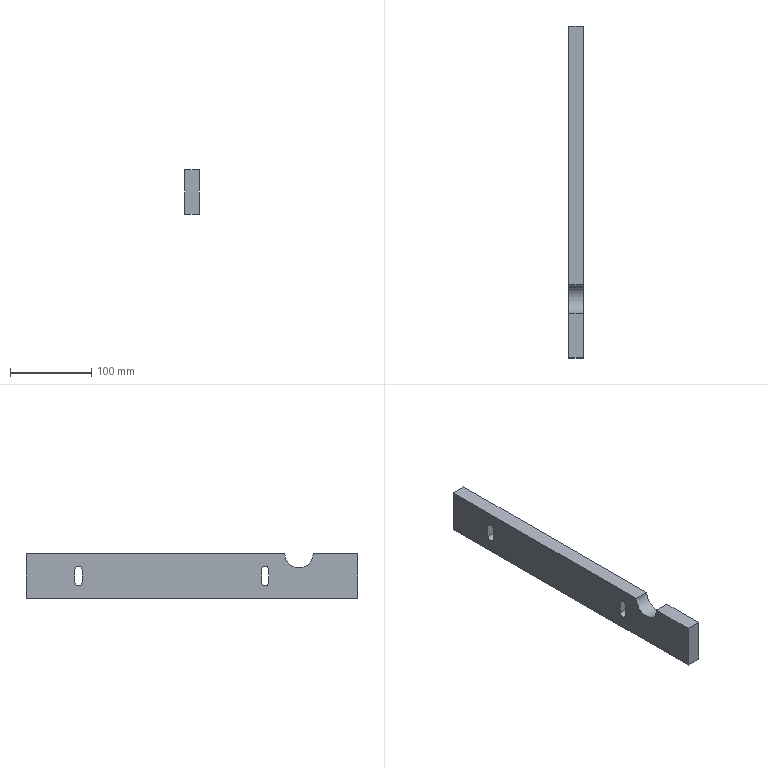Part | STEP file | Superstructure_3 | 1 solid | 16 faces | box 18 x 408 x 55 mm | volume 388111 mm3 | plane 11 | cylinder 5 | commonest cylinder face diameters 9 x4 35 x1
STEP:
#1=CARTESIAN_POINT('',(0.,0.,0.));
#2=DIRECTION('',(0.,0.,1.));
#3=DIRECTION('',(1.,0.,0.));
#4=AXIS2_PLACEMENT_3D('',#1,#2,#3);
#5=CARTESIAN_POINT('',(-9.,204.,27.5));
#6=VERTEX_POINT('',#5);
#7=CARTESIAN_POINT('',(-9.,204.,-27.5));
#8=VERTEX_POINT('',#7);
#9=CARTESIAN_POINT('',(-9.,204.,27.5));
#10=DIRECTION('',(0.,0.,-1.));
#11=VECTOR('',#10,1.);
#12=LINE('',#9,#11);
#13=CARTESIAN_POINT('',(-9.,204.,27.5));
#14=DIRECTION('',(1.,0.,0.));
#15=DIRECTION('',(0.,0.,-1.));
#16=AXIS2_PLACEMENT_3D('',#13,#14,#15);
#17=PLANE('',#16);
#18=CARTESIAN_POINT('',(0.,0.));
#19=DIRECTION('',(1.,0.));
#20=VECTOR('',#19,1.);
#21=LINE('',#18,#20);
#22=(GEOMETRIC_REPRESENTATION_CONTEXT(2)PARAMETRIC_REPRESENTATION_CONTEXT()REPRESENTATION_CONTEXT('',''));
#23=DEFINITIONAL_REPRESENTATION('',(#21),#22);
#24=PCURVE('',#17,#23);
#25=CARTESIAN_POINT('',(0.,204.,0.));
#26=DIRECTION('',(0.,1.,0.));
#27=DIRECTION('',(0.,0.,1.));
#28=AXIS2_PLACEMENT_3D('',#25,#26,#27);
#29=PLANE('',#28);
#30=CARTESIAN_POINT('',(27.5,-9.));
#31=DIRECTION('',(-1.,0.));
#32=VECTOR('',#31,1.);
#33=LINE('',#30,#32);
#34=(GEOMETRIC_REPRESENTATION_CONTEXT(2)PARAMETRIC_REPRESENTATION_CONTEXT()REPRESENTATION_CONTEXT('',''));
#35=DEFINITIONAL_REPRESENTATION('',(#33),#34);
#36=PCURVE('',#29,#35);
#37=SURFACE_CURVE('',#12,(#24,#36),.PCURVE_S1.);
#38=EDGE_CURVE('',#6,#8,#37,.T.);
#39=ORIENTED_EDGE('',*,*,#38,.F.);
#40=CARTESIAN_POINT('',(-9.,-114.,27.5));
#41=VERTEX_POINT('',#40);
#42=CARTESIAN_POINT('',(-9.,204.,27.5));
#43=DIRECTION('',(0.,-1.,0.));
#44=VECTOR('',#43,1.);
#45=LINE('',#42,#44);
#46=CARTESIAN_POINT('',(0.,0.));
#47=DIRECTION('',(0.,-1.));
#48=VECTOR('',#47,1.);
#49=LINE('',#46,#48);
#50=(GEOMETRIC_REPRESENTATION_CONTEXT(2)PARAMETRIC_REPRESENTATION_CONTEXT()REPRESENTATION_CONTEXT('',''));
#51=DEFINITIONAL_REPRESENTATION('',(#49),#50);
#52=PCURVE('',#17,#51);
#53=CARTESIAN_POINT('',(9.,204.,27.5));
#54=DIRECTION('',(0.,0.,-1.));
#55=DIRECTION('',(-1.,0.,0.));
#56=AXIS2_PLACEMENT_3D('',#53,#54,#55);
#57=PLANE('',#56);
#58=CARTESIAN_POINT('',(18.,0.));
#59=DIRECTION('',(0.,-1.));
#60=VECTOR('',#59,1.);
#61=LINE('',#58,#60);
#62=(GEOMETRIC_REPRESENTATION_CONTEXT(2)PARAMETRIC_REPRESENTATION_CONTEXT()REPRESENTATION_CONTEXT('',''));
#63=DEFINITIONAL_REPRESENTATION('',(#61),#62);
#64=PCURVE('',#57,#63);
#65=SURFACE_CURVE('',#45,(#52,#64),.PCURVE_S1.);
#66=EDGE_CURVE('',#6,#41,#65,.T.);
#67=ORIENTED_EDGE('',*,*,#66,.T.);
#68=CARTESIAN_POINT('',(-9.,-149.,27.5));
#69=VERTEX_POINT('',#68);
#70=CARTESIAN_POINT('',(-9.,-131.5,27.5));
#71=DIRECTION('',(1.,0.,0.));
#72=DIRECTION('',(0.,1.,0.));
#73=AXIS2_PLACEMENT_3D('',#70,#71,#72);
#74=CIRCLE('',#73,17.5);
#75=CARTESIAN_POINT('',(0.,-335.5));
#76=DIRECTION('',(0.,1.));
#77=AXIS2_PLACEMENT_2D('',#75,#76);
#78=CIRCLE('',#77,17.5);
#79=(GEOMETRIC_REPRESENTATION_CONTEXT(2)PARAMETRIC_REPRESENTATION_CONTEXT()REPRESENTATION_CONTEXT('',''));
#80=DEFINITIONAL_REPRESENTATION('',(#78),#79);
#81=PCURVE('',#17,#80);
#82=CARTESIAN_POINT('',(15.,-131.5,27.5));
#83=DIRECTION('',(1.,0.,0.));
#84=DIRECTION('',(0.,1.,0.));
#85=AXIS2_PLACEMENT_3D('',#82,#83,#84);
#86=CYLINDRICAL_SURFACE('',#85,17.5);
#87=CARTESIAN_POINT('',(0.,-24.));
#88=DIRECTION('',(1.,0.));
#89=VECTOR('',#88,1.);
#90=LINE('',#87,#89);
#91=(GEOMETRIC_REPRESENTATION_CONTEXT(2)PARAMETRIC_REPRESENTATION_CONTEXT()REPRESENTATION_CONTEXT('',''));
#92=DEFINITIONAL_REPRESENTATION('',(#90),#91);
#93=PCURVE('',#86,#92);
#94=SURFACE_CURVE('',#74,(#81,#93),.PCURVE_S1.);
#95=EDGE_CURVE('',#69,#41,#94,.T.);
#96=ORIENTED_EDGE('',*,*,#95,.F.);
#97=CARTESIAN_POINT('',(-9.,-204.,27.5));
#98=VERTEX_POINT('',#97);
#99=CARTESIAN_POINT('',(-9.,204.,27.5));
#100=DIRECTION('',(0.,-1.,0.));
#101=VECTOR('',#100,1.);
#102=LINE('',#99,#101);
#103=CARTESIAN_POINT('',(0.,0.));
#104=DIRECTION('',(0.,-1.));
#105=VECTOR('',#104,1.);
#106=LINE('',#103,#105);
#107=(GEOMETRIC_REPRESENTATION_CONTEXT(2)PARAMETRIC_REPRESENTATION_CONTEXT()REPRESENTATION_CONTEXT('',''));
#108=DEFINITIONAL_REPRESENTATION('',(#106),#107);
#109=PCURVE('',#17,#108);
#110=CARTESIAN_POINT('',(9.,204.,27.5));
#111=DIRECTION('',(0.,0.,-1.));
#112=DIRECTION('',(-1.,0.,0.));
#113=AXIS2_PLACEMENT_3D('',#110,#111,#112);
#114=PLANE('',#113);
#115=CARTESIAN_POINT('',(18.,0.));
#116=DIRECTION('',(0.,-1.));
#117=VECTOR('',#116,1.);
#118=LINE('',#115,#117);
#119=(GEOMETRIC_REPRESENTATION_CONTEXT(2)PARAMETRIC_REPRESENTATION_CONTEXT()REPRESENTATION_CONTEXT('',''));
#120=DEFINITIONAL_REPRESENTATION('',(#118),#119);
#121=PCURVE('',#114,#120);
#122=SURFACE_CURVE('',#102,(#109,#121),.PCURVE_S1.);
#123=EDGE_CURVE('',#69,#98,#122,.T.);
#124=ORIENTED_EDGE('',*,*,#123,.T.);
#125=CARTESIAN_POINT('',(-9.,-204.,-27.5));
#126=VERTEX_POINT('',#125);
#127=CARTESIAN_POINT('',(-9.,-204.,27.5));
#128=DIRECTION('',(0.,0.,-1.));
#129=VECTOR('',#128,1.);
#130=LINE('',#127,#129);
#131=CARTESIAN_POINT('',(0.,-408.));
#132=DIRECTION('',(1.,0.));
#133=VECTOR('',#132,1.);
#134=LINE('',#131,#133);
#135=(GEOMETRIC_REPRESENTATION_CONTEXT(2)PARAMETRIC_REPRESENTATION_CONTEXT()REPRESENTATION_CONTEXT('',''));
#136=DEFINITIONAL_REPRESENTATION('',(#134),#135);
#137=PCURVE('',#17,#136);
#138=CARTESIAN_POINT('',(0.,-204.,0.));
#139=DIRECTION('',(0.,1.,0.));
#140=DIRECTION('',(0.,0.,1.));
#141=AXIS2_PLACEMENT_3D('',#138,#139,#140);
#142=PLANE('',#141);
#143=CARTESIAN_POINT('',(27.5,-9.));
#144=DIRECTION('',(-1.,0.));
#145=VECTOR('',#144,1.);
#146=LINE('',#143,#145);
#147=(GEOMETRIC_REPRESENTATION_CONTEXT(2)PARAMETRIC_REPRESENTATION_CONTEXT()REPRESENTATION_CONTEXT('',''));
#148=DEFINITIONAL_REPRESENTATION('',(#146),#147);
#149=PCURVE('',#142,#148);
#150=SURFACE_CURVE('',#130,(#137,#149),.PCURVE_S1.);
#151=EDGE_CURVE('',#98,#126,#150,.T.);
#152=ORIENTED_EDGE('',*,*,#151,.T.);
#153=CARTESIAN_POINT('',(-9.,204.,-27.5));
#154=DIRECTION('',(0.,-1.,0.));
#155=VECTOR('',#154,1.);
#156=LINE('',#153,#155);
#157=CARTESIAN_POINT('',(55.,0.));
#158=DIRECTION('',(0.,-1.));
#159=VECTOR('',#158,1.);
#160=LINE('',#157,#159);
#161=(GEOMETRIC_REPRESENTATION_CONTEXT(2)PARAMETRIC_REPRESENTATION_CONTEXT()REPRESENTATION_CONTEXT('',''));
#162=DEFINITIONAL_REPRESENTATION('',(#160),#161);
#163=PCURVE('',#17,#162);
#164=CARTESIAN_POINT('',(-9.,204.,-27.5));
#165=DIRECTION('',(0.,0.,1.));
#166=DIRECTION('',(1.,0.,0.));
#167=AXIS2_PLACEMENT_3D('',#164,#165,#166);
#168=PLANE('',#167);
#169=CARTESIAN_POINT('',(0.,0.));
#170=DIRECTION('',(0.,-1.));
#171=VECTOR('',#170,1.);
#172=LINE('',#169,#171);
#173=(GEOMETRIC_REPRESENTATION_CONTEXT(2)PARAMETRIC_REPRESENTATION_CONTEXT()REPRESENTATION_CONTEXT('',''));
#174=DEFINITIONAL_REPRESENTATION('',(#172),#173);
#175=PCURVE('',#168,#174);
#176=SURFACE_CURVE('',#156,(#163,#175),.PCURVE_S1.);
#177=EDGE_CURVE('',#8,#126,#176,.T.);
#178=ORIENTED_EDGE('',*,*,#177,.F.);
#179=EDGE_LOOP('',(#39,#67,#96,#124,#152,#178));
#180=FACE_BOUND('',#179,.F.);
#181=CARTESIAN_POINT('',(-9.,-85.5,7.5));
#182=VERTEX_POINT('',#181);
#183=CARTESIAN_POINT('',(-9.,-94.5,7.5));
#184=VERTEX_POINT('',#183);
#185=CARTESIAN_POINT('',(-9.,-90.,7.5));
#186=DIRECTION('',(1.,0.,0.));
#187=DIRECTION('',(0.,1.,0.));
#188=AXIS2_PLACEMENT_3D('',#185,#186,#187);
#189=CIRCLE('',#188,4.5);
#190=CARTESIAN_POINT('',(20.,-294.));
#191=DIRECTION('',(0.,1.));
#192=AXIS2_PLACEMENT_2D('',#190,#191);
#193=CIRCLE('',#192,4.5);
#194=(GEOMETRIC_REPRESENTATION_CONTEXT(2)PARAMETRIC_REPRESENTATION_CONTEXT()REPRESENTATION_CONTEXT('',''));
#195=DEFINITIONAL_REPRESENTATION('',(#193),#194);
#196=PCURVE('',#17,#195);
#197=CARTESIAN_POINT('',(10.,-90.,7.5));
#198=DIRECTION('',(1.,0.,0.));
#199=DIRECTION('',(0.,1.,0.));
#200=AXIS2_PLACEMENT_3D('',#197,#198,#199);
#201=CYLINDRICAL_SURFACE('',#200,4.5);
#202=CARTESIAN_POINT('',(0.,-19.));
#203=DIRECTION('',(1.,0.));
#204=VECTOR('',#203,1.);
#205=LINE('',#202,#204);
#206=(GEOMETRIC_REPRESENTATION_CONTEXT(2)PARAMETRIC_REPRESENTATION_CONTEXT()REPRESENTATION_CONTEXT('',''));
#207=DEFINITIONAL_REPRESENTATION('',(#205),#206);
#208=PCURVE('',#201,#207);
#209=SURFACE_CURVE('',#189,(#196,#208),.PCURVE_S1.);
#210=EDGE_CURVE('',#182,#184,#209,.T.);
#211=ORIENTED_EDGE('',*,*,#210,.F.);
#212=CARTESIAN_POINT('',(-9.,-85.5,-7.5));
#213=VERTEX_POINT('',#212);
#214=CARTESIAN_POINT('',(-9.,-85.5,17.5));
#215=DIRECTION('',(0.,0.,-1.));
#216=VECTOR('',#215,1.);
#217=LINE('',#214,#216);
#218=CARTESIAN_POINT('',(10.,-289.5));
#219=DIRECTION('',(1.,0.));
#220=VECTOR('',#219,1.);
#221=LINE('',#218,#220);
#222=(GEOMETRIC_REPRESENTATION_CONTEXT(2)PARAMETRIC_REPRESENTATION_CONTEXT()REPRESENTATION_CONTEXT('',''));
#223=DEFINITIONAL_REPRESENTATION('',(#221),#222);
#224=PCURVE('',#17,#223);
#225=CARTESIAN_POINT('',(10.,-85.5,7.5));
#226=DIRECTION('',(0.,-1.,0.));
#227=DIRECTION('',(0.,0.,-1.));
#228=AXIS2_PLACEMENT_3D('',#225,#226,#227);
#229=PLANE('',#228);
#230=CARTESIAN_POINT('',(-10.,-19.));
#231=DIRECTION('',(1.,0.));
#232=VECTOR('',#231,1.);
#233=LINE('',#230,#232);
#234=(GEOMETRIC_REPRESENTATION_CONTEXT(2)PARAMETRIC_REPRESENTATION_CONTEXT()REPRESENTATION_CONTEXT('',''));
#235=DEFINITIONAL_REPRESENTATION('',(#233),#234);
#236=PCURVE('',#229,#235);
#237=SURFACE_CURVE('',#217,(#224,#236),.PCURVE_S1.);
#238=EDGE_CURVE('',#182,#213,#237,.T.);
#239=ORIENTED_EDGE('',*,*,#238,.T.);
#240=CARTESIAN_POINT('',(-9.,-94.5,-7.5));
#241=VERTEX_POINT('',#240);
#242=CARTESIAN_POINT('',(-9.,-90.,-7.5));
#243=DIRECTION('',(1.,0.,0.));
#244=DIRECTION('',(0.,1.,0.));
#245=AXIS2_PLACEMENT_3D('',#242,#243,#244);
#246=CIRCLE('',#245,4.5);
#247=CARTESIAN_POINT('',(35.,-294.));
#248=DIRECTION('',(0.,1.));
#249=AXIS2_PLACEMENT_2D('',#247,#248);
#250=CIRCLE('',#249,4.5);
#251=(GEOMETRIC_REPRESENTATION_CONTEXT(2)PARAMETRIC_REPRESENTATION_CONTEXT()REPRESENTATION_CONTEXT('',''));
#252=DEFINITIONAL_REPRESENTATION('',(#250),#251);
#253=PCURVE('',#17,#252);
#254=CARTESIAN_POINT('',(10.,-90.,-7.5));
#255=DIRECTION('',(1.,0.,0.));
#256=DIRECTION('',(0.,1.,0.));
#257=AXIS2_PLACEMENT_3D('',#254,#255,#256);
#258=CYLINDRICAL_SURFACE('',#257,4.5);
#259=CARTESIAN_POINT('',(0.,-19.));
#260=DIRECTION('',(1.,0.));
#261=VECTOR('',#260,1.);
#262=LINE('',#259,#261);
#263=(GEOMETRIC_REPRESENTATION_CONTEXT(2)PARAMETRIC_REPRESENTATION_CONTEXT()REPRESENTATION_CONTEXT('',''));
#264=DEFINITIONAL_REPRESENTATION('',(#262),#263);
#265=PCURVE('',#258,#264);
#266=SURFACE_CURVE('',#246,(#253,#265),.PCURVE_S1.);
#267=EDGE_CURVE('',#241,#213,#266,.T.);
#268=ORIENTED_EDGE('',*,*,#267,.F.);
#269=CARTESIAN_POINT('',(-9.,-94.5,17.5));
#270=DIRECTION('',(0.,0.,-1.));
#271=VECTOR('',#270,1.);
#272=LINE('',#269,#271);
#273=CARTESIAN_POINT('',(10.,-298.5));
#274=DIRECTION('',(1.,0.));
#275=VECTOR('',#274,1.);
#276=LINE('',#273,#275);
#277=(GEOMETRIC_REPRESENTATION_CONTEXT(2)PARAMETRIC_REPRESENTATION_CONTEXT()REPRESENTATION_CONTEXT('',''));
#278=DEFINITIONAL_REPRESENTATION('',(#276),#277);
#279=PCURVE('',#17,#278);
#280=CARTESIAN_POINT('',(10.,-94.5,7.5));
#281=DIRECTION('',(0.,-1.,0.));
#282=DIRECTION('',(0.,0.,-1.));
#283=AXIS2_PLACEMENT_3D('',#280,#281,#282);
#284=PLANE('',#283);
#285=CARTESIAN_POINT('',(-10.,-19.));
#286=DIRECTION('',(1.,0.));
#287=VECTOR('',#286,1.);
#288=LINE('',#285,#287);
#289=(GEOMETRIC_REPRESENTATION_CONTEXT(2)PARAMETRIC_REPRESENTATION_CONTEXT()REPRESENTATION_CONTEXT('',''));
#290=DEFINITIONAL_REPRESENTATION('',(#288),#289);
#291=PCURVE('',#284,#290);
#292=SURFACE_CURVE('',#272,(#279,#291),.PCURVE_S1.);
#293=EDGE_CURVE('',#184,#241,#292,.T.);
#294=ORIENTED_EDGE('',*,*,#293,.F.);
#295=EDGE_LOOP('',(#211,#239,#268,#294));
#296=FACE_BOUND('',#295,.F.);
#297=CARTESIAN_POINT('',(-9.,144.,7.5));
#298=VERTEX_POINT('',#297);
#299=CARTESIAN_POINT('',(-9.,135.,7.5));
#300=VERTEX_POINT('',#299);
#301=CARTESIAN_POINT('',(-9.,139.5,7.5));
#302=DIRECTION('',(1.,0.,0.));
#303=DIRECTION('',(0.,1.,0.));
#304=AXIS2_PLACEMENT_3D('',#301,#302,#303);
#305=CIRCLE('',#304,4.5);
#306=CARTESIAN_POINT('',(20.,-64.5));
#307=DIRECTION('',(0.,1.));
#308=AXIS2_PLACEMENT_2D('',#306,#307);
#309=CIRCLE('',#308,4.5);
#310=(GEOMETRIC_REPRESENTATION_CONTEXT(2)PARAMETRIC_REPRESENTATION_CONTEXT()REPRESENTATION_CONTEXT('',''));
#311=DEFINITIONAL_REPRESENTATION('',(#309),#310);
#312=PCURVE('',#17,#311);
#313=CARTESIAN_POINT('',(10.,139.5,7.5));
#314=DIRECTION('',(1.,0.,0.));
#315=DIRECTION('',(0.,1.,0.));
#316=AXIS2_PLACEMENT_3D('',#313,#314,#315);
#317=CYLINDRICAL_SURFACE('',#316,4.5);
#318=CARTESIAN_POINT('',(0.,-19.));
#319=DIRECTION('',(1.,0.));
#320=VECTOR('',#319,1.);
#321=LINE('',#318,#320);
#322=(GEOMETRIC_REPRESENTATION_CONTEXT(2)PARAMETRIC_REPRESENTATION_CONTEXT()REPRESENTATION_CONTEXT('',''));
#323=DEFINITIONAL_REPRESENTATION('',(#321),#322);
#324=PCURVE('',#317,#323);
#325=SURFACE_CURVE('',#305,(#312,#324),.PCURVE_S1.);
#326=EDGE_CURVE('',#298,#300,#325,.T.);
#327=ORIENTED_EDGE('',*,*,#326,.F.);
#328=CARTESIAN_POINT('',(-9.,144.,-7.5));
#329=VERTEX_POINT('',#328);
#330=CARTESIAN_POINT('',(-9.,144.,17.5));
#331=DIRECTION('',(0.,0.,-1.));
#332=VECTOR('',#331,1.);
#333=LINE('',#330,#332);
#334=CARTESIAN_POINT('',(10.,-60.));
#335=DIRECTION('',(1.,0.));
#336=VECTOR('',#335,1.);
#337=LINE('',#334,#336);
#338=(GEOMETRIC_REPRESENTATION_CONTEXT(2)PARAMETRIC_REPRESENTATION_CONTEXT()REPRESENTATION_CONTEXT('',''));
#339=DEFINITIONAL_REPRESENTATION('',(#337),#338);
#340=PCURVE('',#17,#339);
#341=CARTESIAN_POINT('',(10.,144.,7.5));
#342=DIRECTION('',(0.,-1.,0.));
#343=DIRECTION('',(0.,0.,-1.));
#344=AXIS2_PLACEMENT_3D('',#341,#342,#343);
#345=PLANE('',#344);
#346=CARTESIAN_POINT('',(-10.,-19.));
#347=DIRECTION('',(1.,0.));
#348=VECTOR('',#347,1.);
#349=LINE('',#346,#348);
#350=(GEOMETRIC_REPRESENTATION_CONTEXT(2)PARAMETRIC_REPRESENTATION_CONTEXT()REPRESENTATION_CONTEXT('',''));
#351=DEFINITIONAL_REPRESENTATION('',(#349),#350);
#352=PCURVE('',#345,#351);
#353=SURFACE_CURVE('',#333,(#340,#352),.PCURVE_S1.);
#354=EDGE_CURVE('',#298,#329,#353,.T.);
#355=ORIENTED_EDGE('',*,*,#354,.T.);
#356=CARTESIAN_POINT('',(-9.,135.,-7.5));
#357=VERTEX_POINT('',#356);
#358=CARTESIAN_POINT('',(-9.,139.5,-7.5));
#359=DIRECTION('',(1.,0.,0.));
#360=DIRECTION('',(0.,1.,0.));
#361=AXIS2_PLACEMENT_3D('',#358,#359,#360);
#362=CIRCLE('',#361,4.5);
#363=CARTESIAN_POINT('',(35.,-64.5));
#364=DIRECTION('',(0.,1.));
#365=AXIS2_PLACEMENT_2D('',#363,#364);
#366=CIRCLE('',#365,4.5);
#367=(GEOMETRIC_REPRESENTATION_CONTEXT(2)PARAMETRIC_REPRESENTATION_CONTEXT()REPRESENTATION_CONTEXT('',''));
#368=DEFINITIONAL_REPRESENTATION('',(#366),#367);
#369=PCURVE('',#17,#368);
#370=CARTESIAN_POINT('',(10.,139.5,-7.5));
#371=DIRECTION('',(1.,0.,0.));
#372=DIRECTION('',(0.,1.,0.));
#373=AXIS2_PLACEMENT_3D('',#370,#371,#372);
#374=CYLINDRICAL_SURFACE('',#373,4.5);
#375=CARTESIAN_POINT('',(0.,-19.));
#376=DIRECTION('',(1.,0.));
#377=VECTOR('',#376,1.);
#378=LINE('',#375,#377);
#379=(GEOMETRIC_REPRESENTATION_CONTEXT(2)PARAMETRIC_REPRESENTATION_CONTEXT()REPRESENTATION_CONTEXT('',''));
#380=DEFINITIONAL_REPRESENTATION('',(#378),#379);
#381=PCURVE('',#374,#380);
#382=SURFACE_CURVE('',#362,(#369,#381),.PCURVE_S1.);
#383=EDGE_CURVE('',#357,#329,#382,.T.);
#384=ORIENTED_EDGE('',*,*,#383,.F.);
#385=CARTESIAN_POINT('',(-9.,135.,17.5));
#386=DIRECTION('',(0.,0.,-1.));
#387=VECTOR('',#386,1.);
#388=LINE('',#385,#387);
#389=CARTESIAN_POINT('',(10.,-69.));
#390=DIRECTION('',(1.,0.));
#391=VECTOR('',#390,1.);
#392=LINE('',#389,#391);
#393=(GEOMETRIC_REPRESENTATION_CONTEXT(2)PARAMETRIC_REPRESENTATION_CONTEXT()REPRESENTATION_CONTEXT('',''));
#394=DEFINITIONAL_REPRESENTATION('',(#392),#393);
#395=PCURVE('',#17,#394);
#396=CARTESIAN_POINT('',(10.,135.,7.5));
#397=DIRECTION('',(0.,-1.,0.));
#398=DIRECTION('',(0.,0.,-1.));
#399=AXIS2_PLACEMENT_3D('',#396,#397,#398);
#400=PLANE('',#399);
#401=CARTESIAN_POINT('',(-10.,-19.));
#402=DIRECTION('',(1.,0.));
#403=VECTOR('',#402,1.);
#404=LINE('',#401,#403);
#405=(GEOMETRIC_REPRESENTATION_CONTEXT(2)PARAMETRIC_REPRESENTATION_CONTEXT()REPRESENTATION_CONTEXT('',''));
#406=DEFINITIONAL_REPRESENTATION('',(#404),#405);
#407=PCURVE('',#400,#406);
#408=SURFACE_CURVE('',#388,(#395,#407),.PCURVE_S1.);
#409=EDGE_CURVE('',#300,#357,#408,.T.);
#410=ORIENTED_EDGE('',*,*,#409,.F.);
#411=EDGE_LOOP('',(#327,#355,#384,#410));
#412=FACE_BOUND('',#411,.F.);
#413=ADVANCED_FACE('',(#180,#296,#412),#17,.F.);
#414=ORIENTED_EDGE('',*,*,#38,.T.);
#415=CARTESIAN_POINT('',(9.,204.,-27.5));
#416=VERTEX_POINT('',#415);
#417=CARTESIAN_POINT('',(-9.,204.,-27.5));
#418=DIRECTION('',(1.,0.,0.));
#419=VECTOR('',#418,1.);
#420=LINE('',#417,#419);
#421=CARTESIAN_POINT('',(-27.5,-9.));
#422=DIRECTION('',(0.,1.));
#423=VECTOR('',#422,1.);
#424=LINE('',#421,#423);
#425=(GEOMETRIC_REPRESENTATION_CONTEXT(2)PARAMETRIC_REPRESENTATION_CONTEXT()REPRESENTATION_CONTEXT('',''));
#426=DEFINITIONAL_REPRESENTATION('',(#424),#425);
#427=PCURVE('',#29,#426);
#428=CARTESIAN_POINT('',(0.,0.));
#429=DIRECTION('',(1.,0.));
#430=VECTOR('',#429,1.);
#431=LINE('',#428,#430);
#432=(GEOMETRIC_REPRESENTATION_CONTEXT(2)PARAMETRIC_REPRESENTATION_CONTEXT()REPRESENTATION_CONTEXT('',''));
#433=DEFINITIONAL_REPRESENTATION('',(#431),#432);
#434=PCURVE('',#168,#433);
#435=SURFACE_CURVE('',#420,(#427,#434),.PCURVE_S1.);
#436=EDGE_CURVE('',#8,#416,#435,.T.);
#437=ORIENTED_EDGE('',*,*,#436,.T.);
#438=CARTESIAN_POINT('',(9.,204.,27.5));
#439=VERTEX_POINT('',#438);
#440=CARTESIAN_POINT('',(9.,204.,-27.5));
#441=DIRECTION('',(0.,0.,1.));
#442=VECTOR('',#441,1.);
#443=LINE('',#440,#442);
#444=CARTESIAN_POINT('',(-27.5,9.));
#445=DIRECTION('',(1.,0.));
#446=VECTOR('',#445,1.);
#447=LINE('',#444,#446);
#448=(GEOMETRIC_REPRESENTATION_CONTEXT(2)PARAMETRIC_REPRESENTATION_CONTEXT()REPRESENTATION_CONTEXT('',''));
#449=DEFINITIONAL_REPRESENTATION('',(#447),#448);
#450=PCURVE('',#29,#449);
#451=CARTESIAN_POINT('',(9.,204.,-27.5));
#452=DIRECTION('',(-1.,0.,0.));
#453=DIRECTION('',(0.,0.,1.));
#454=AXIS2_PLACEMENT_3D('',#451,#452,#453);
#455=PLANE('',#454);
#456=CARTESIAN_POINT('',(0.,0.));
#457=DIRECTION('',(1.,0.));
#458=VECTOR('',#457,1.);
#459=LINE('',#456,#458);
#460=(GEOMETRIC_REPRESENTATION_CONTEXT(2)PARAMETRIC_REPRESENTATION_CONTEXT()REPRESENTATION_CONTEXT('',''));
#461=DEFINITIONAL_REPRESENTATION('',(#459),#460);
#462=PCURVE('',#455,#461);
#463=SURFACE_CURVE('',#443,(#450,#462),.PCURVE_S1.);
#464=EDGE_CURVE('',#416,#439,#463,.T.);
#465=ORIENTED_EDGE('',*,*,#464,.T.);
#466=CARTESIAN_POINT('',(9.,204.,27.5));
#467=DIRECTION('',(-1.,0.,0.));
#468=VECTOR('',#467,1.);
#469=LINE('',#466,#468);
#470=CARTESIAN_POINT('',(27.5,9.));
#471=DIRECTION('',(0.,-1.));
#472=VECTOR('',#471,1.);
#473=LINE('',#470,#472);
#474=(GEOMETRIC_REPRESENTATION_CONTEXT(2)PARAMETRIC_REPRESENTATION_CONTEXT()REPRESENTATION_CONTEXT('',''));
#475=DEFINITIONAL_REPRESENTATION('',(#473),#474);
#476=PCURVE('',#29,#475);
#477=CARTESIAN_POINT('',(0.,0.));
#478=DIRECTION('',(1.,0.));
#479=VECTOR('',#478,1.);
#480=LINE('',#477,#479);
#481=(GEOMETRIC_REPRESENTATION_CONTEXT(2)PARAMETRIC_REPRESENTATION_CONTEXT()REPRESENTATION_CONTEXT('',''));
#482=DEFINITIONAL_REPRESENTATION('',(#480),#481);
#483=PCURVE('',#57,#482);
#484=SURFACE_CURVE('',#469,(#476,#483),.PCURVE_S1.);
#485=EDGE_CURVE('',#439,#6,#484,.T.);
#486=ORIENTED_EDGE('',*,*,#485,.T.);
#487=EDGE_LOOP('',(#414,#437,#465,#486));
#488=FACE_BOUND('',#487,.F.);
#489=ADVANCED_FACE('',(#488),#29,.T.);
#490=ORIENTED_EDGE('',*,*,#177,.T.);
#491=CARTESIAN_POINT('',(9.,-204.,-27.5));
#492=VERTEX_POINT('',#491);
#493=CARTESIAN_POINT('',(-9.,-204.,-27.5));
#494=DIRECTION('',(1.,0.,0.));
#495=VECTOR('',#494,1.);
#496=LINE('',#493,#495);
#497=CARTESIAN_POINT('',(0.,-408.));
#498=DIRECTION('',(1.,0.));
#499=VECTOR('',#498,1.);
#500=LINE('',#497,#499);
#501=(GEOMETRIC_REPRESENTATION_CONTEXT(2)PARAMETRIC_REPRESENTATION_CONTEXT()REPRESENTATION_CONTEXT('',''));
#502=DEFINITIONAL_REPRESENTATION('',(#500),#501);
#503=PCURVE('',#168,#502);
#504=CARTESIAN_POINT('',(-27.5,-9.));
#505=DIRECTION('',(0.,1.));
#506=VECTOR('',#505,1.);
#507=LINE('',#504,#506);
#508=(GEOMETRIC_REPRESENTATION_CONTEXT(2)PARAMETRIC_REPRESENTATION_CONTEXT()REPRESENTATION_CONTEXT('',''));
#509=DEFINITIONAL_REPRESENTATION('',(#507),#508);
#510=PCURVE('',#142,#509);
#511=SURFACE_CURVE('',#496,(#503,#510),.PCURVE_S1.);
#512=EDGE_CURVE('',#126,#492,#511,.T.);
#513=ORIENTED_EDGE('',*,*,#512,.T.);
#514=CARTESIAN_POINT('',(9.,204.,-27.5));
#515=DIRECTION('',(0.,-1.,0.));
#516=VECTOR('',#515,1.);
#517=LINE('',#514,#516);
#518=CARTESIAN_POINT('',(18.,0.));
#519=DIRECTION('',(0.,-1.));
#520=VECTOR('',#519,1.);
#521=LINE('',#518,#520);
#522=(GEOMETRIC_REPRESENTATION_CONTEXT(2)PARAMETRIC_REPRESENTATION_CONTEXT()REPRESENTATION_CONTEXT('',''));
#523=DEFINITIONAL_REPRESENTATION('',(#521),#522);
#524=PCURVE('',#168,#523);
#525=CARTESIAN_POINT('',(0.,0.));
#526=DIRECTION('',(0.,-1.));
#527=VECTOR('',#526,1.);
#528=LINE('',#525,#527);
#529=(GEOMETRIC_REPRESENTATION_CONTEXT(2)PARAMETRIC_REPRESENTATION_CONTEXT()REPRESENTATION_CONTEXT('',''));
#530=DEFINITIONAL_REPRESENTATION('',(#528),#529);
#531=PCURVE('',#455,#530);
#532=SURFACE_CURVE('',#517,(#524,#531),.PCURVE_S1.);
#533=EDGE_CURVE('',#416,#492,#532,.T.);
#534=ORIENTED_EDGE('',*,*,#533,.F.);
#535=ORIENTED_EDGE('',*,*,#436,.F.);
#536=EDGE_LOOP('',(#490,#513,#534,#535));
#537=FACE_BOUND('',#536,.F.);
#538=ADVANCED_FACE('',(#537),#168,.F.);
#539=ORIENTED_EDGE('',*,*,#151,.T.);
#540=ORIENTED_EDGE('',*,*,#512,.T.);
#541=CARTESIAN_POINT('',(9.,-204.,27.5));
#542=VERTEX_POINT('',#541);
#543=CARTESIAN_POINT('',(9.,-204.,-27.5));
#544=DIRECTION('',(0.,0.,1.));
#545=VECTOR('',#544,1.);
#546=LINE('',#543,#545);
#547=CARTESIAN_POINT('',(-27.5,9.));
#548=DIRECTION('',(1.,0.));
#549=VECTOR('',#548,1.);
#550=LINE('',#547,#549);
#551=(GEOMETRIC_REPRESENTATION_CONTEXT(2)PARAMETRIC_REPRESENTATION_CONTEXT()REPRESENTATION_CONTEXT('',''));
#552=DEFINITIONAL_REPRESENTATION('',(#550),#551);
#553=PCURVE('',#142,#552);
#554=CARTESIAN_POINT('',(0.,-408.));
#555=DIRECTION('',(1.,0.));
#556=VECTOR('',#555,1.);
#557=LINE('',#554,#556);
#558=(GEOMETRIC_REPRESENTATION_CONTEXT(2)PARAMETRIC_REPRESENTATION_CONTEXT()REPRESENTATION_CONTEXT('',''));
#559=DEFINITIONAL_REPRESENTATION('',(#557),#558);
#560=PCURVE('',#455,#559);
#561=SURFACE_CURVE('',#546,(#553,#560),.PCURVE_S1.);
#562=EDGE_CURVE('',#492,#542,#561,.T.);
#563=ORIENTED_EDGE('',*,*,#562,.T.);
#564=CARTESIAN_POINT('',(9.,-204.,27.5));
#565=DIRECTION('',(-1.,0.,0.));
#566=VECTOR('',#565,1.);
#567=LINE('',#564,#566);
#568=CARTESIAN_POINT('',(27.5,9.));
#569=DIRECTION('',(0.,-1.));
#570=VECTOR('',#569,1.);
#571=LINE('',#568,#570);
#572=(GEOMETRIC_REPRESENTATION_CONTEXT(2)PARAMETRIC_REPRESENTATION_CONTEXT()REPRESENTATION_CONTEXT('',''));
#573=DEFINITIONAL_REPRESENTATION('',(#571),#572);
#574=PCURVE('',#142,#573);
#575=CARTESIAN_POINT('',(0.,-408.));
#576=DIRECTION('',(1.,0.));
#577=VECTOR('',#576,1.);
#578=LINE('',#575,#577);
#579=(GEOMETRIC_REPRESENTATION_CONTEXT(2)PARAMETRIC_REPRESENTATION_CONTEXT()REPRESENTATION_CONTEXT('',''));
#580=DEFINITIONAL_REPRESENTATION('',(#578),#579);
#581=PCURVE('',#114,#580);
#582=SURFACE_CURVE('',#567,(#574,#581),.PCURVE_S1.);
#583=EDGE_CURVE('',#542,#98,#582,.T.);
#584=ORIENTED_EDGE('',*,*,#583,.T.);
#585=EDGE_LOOP('',(#539,#540,#563,#584));
#586=FACE_BOUND('',#585,.T.);
#587=ADVANCED_FACE('',(#586),#142,.F.);
#588=CARTESIAN_POINT('',(9.,-149.,27.5));
#589=VERTEX_POINT('',#588);
#590=CARTESIAN_POINT('',(15.,-149.,27.5));
#591=DIRECTION('',(1.,0.,0.));
#592=VECTOR('',#591,1.);
#593=LINE('',#590,#592);
#594=CARTESIAN_POINT('',(-6.,-353.));
#595=DIRECTION('',(-1.,0.));
#596=VECTOR('',#595,1.);
#597=LINE('',#594,#596);
#598=(GEOMETRIC_REPRESENTATION_CONTEXT(2)PARAMETRIC_REPRESENTATION_CONTEXT()REPRESENTATION_CONTEXT('',''));
#599=DEFINITIONAL_REPRESENTATION('',(#597),#598);
#600=PCURVE('',#114,#599);
#601=CARTESIAN_POINT('',(3.142,0.));
#602=DIRECTION('',(0.,1.));
#603=VECTOR('',#602,1.);
#604=LINE('',#601,#603);
#605=(GEOMETRIC_REPRESENTATION_CONTEXT(2)PARAMETRIC_REPRESENTATION_CONTEXT()REPRESENTATION_CONTEXT('',''));
#606=DEFINITIONAL_REPRESENTATION('',(#604),#605);
#607=PCURVE('',#86,#606);
#608=SURFACE_CURVE('',#593,(#600,#607),.PCURVE_S1.);
#609=EDGE_CURVE('',#69,#589,#608,.T.);
#610=ORIENTED_EDGE('',*,*,#609,.T.);
#611=CARTESIAN_POINT('',(9.,204.,27.5));
#612=DIRECTION('',(0.,-1.,0.));
#613=VECTOR('',#612,1.);
#614=LINE('',#611,#613);
#615=CARTESIAN_POINT('',(0.,0.));
#616=DIRECTION('',(0.,-1.));
#617=VECTOR('',#616,1.);
#618=LINE('',#615,#617);
#619=(GEOMETRIC_REPRESENTATION_CONTEXT(2)PARAMETRIC_REPRESENTATION_CONTEXT()REPRESENTATION_CONTEXT('',''));
#620=DEFINITIONAL_REPRESENTATION('',(#618),#619);
#621=PCURVE('',#114,#620);
#622=CARTESIAN_POINT('',(55.,0.));
#623=DIRECTION('',(0.,-1.));
#624=VECTOR('',#623,1.);
#625=LINE('',#622,#624);
#626=(GEOMETRIC_REPRESENTATION_CONTEXT(2)PARAMETRIC_REPRESENTATION_CONTEXT()REPRESENTATION_CONTEXT('',''));
#627=DEFINITIONAL_REPRESENTATION('',(#625),#626);
#628=PCURVE('',#455,#627);
#629=SURFACE_CURVE('',#614,(#621,#628),.PCURVE_S1.);
#630=EDGE_CURVE('',#589,#542,#629,.T.);
#631=ORIENTED_EDGE('',*,*,#630,.T.);
#632=ORIENTED_EDGE('',*,*,#583,.T.);
#633=ORIENTED_EDGE('',*,*,#123,.F.);
#634=EDGE_LOOP('',(#610,#631,#632,#633));
#635=FACE_BOUND('',#634,.F.);
#636=ADVANCED_FACE('',(#635),#114,.F.);
#637=CARTESIAN_POINT('',(9.,-114.,27.5));
#638=VERTEX_POINT('',#637);
#639=CARTESIAN_POINT('',(15.,-114.,27.5));
#640=DIRECTION('',(-1.,0.,0.));
#641=VECTOR('',#640,1.);
#642=LINE('',#639,#641);
#643=CARTESIAN_POINT('',(6.283,0.));
#644=DIRECTION('',(0.,-1.));
#645=VECTOR('',#644,1.);
#646=LINE('',#643,#645);
#647=(GEOMETRIC_REPRESENTATION_CONTEXT(2)PARAMETRIC_REPRESENTATION_CONTEXT()REPRESENTATION_CONTEXT('',''));
#648=DEFINITIONAL_REPRESENTATION('',(#646),#647);
#649=PCURVE('',#86,#648);
#650=CARTESIAN_POINT('',(-6.,-318.));
#651=DIRECTION('',(1.,0.));
#652=VECTOR('',#651,1.);
#653=LINE('',#650,#652);
#654=(GEOMETRIC_REPRESENTATION_CONTEXT(2)PARAMETRIC_REPRESENTATION_CONTEXT()REPRESENTATION_CONTEXT('',''));
#655=DEFINITIONAL_REPRESENTATION('',(#653),#654);
#656=PCURVE('',#57,#655);
#657=SURFACE_CURVE('',#642,(#649,#656),.PCURVE_S1.);
#658=EDGE_CURVE('',#638,#41,#657,.T.);
#659=ORIENTED_EDGE('',*,*,#658,.F.);
#660=CARTESIAN_POINT('',(9.,-131.5,27.5));
#661=DIRECTION('',(1.,0.,0.));
#662=DIRECTION('',(0.,1.,0.));
#663=AXIS2_PLACEMENT_3D('',#660,#661,#662);
#664=CIRCLE('',#663,17.5);
#665=CARTESIAN_POINT('',(0.,-6.));
#666=DIRECTION('',(1.,0.));
#667=VECTOR('',#666,1.);
#668=LINE('',#665,#667);
#669=(GEOMETRIC_REPRESENTATION_CONTEXT(2)PARAMETRIC_REPRESENTATION_CONTEXT()REPRESENTATION_CONTEXT('',''));
#670=DEFINITIONAL_REPRESENTATION('',(#668),#669);
#671=PCURVE('',#86,#670);
#672=CARTESIAN_POINT('',(55.,-318.));
#673=CARTESIAN_POINT('',(85.311,-318.));
#674=CARTESIAN_POINT('',(70.155,-344.25));
#675=CARTESIAN_POINT('',(55.,-370.5));
#676=CARTESIAN_POINT('',(39.845,-344.25));
#677=CARTESIAN_POINT('',(24.689,-318.));
#678=CARTESIAN_POINT('',(55.,-318.));
#679=(BOUNDED_CURVE()B_SPLINE_CURVE(2,(#672,#673,#674,#675,#676,#677,#678),.UNSPECIFIED.,.T.,.F.)B_SPLINE_CURVE_WITH_KNOTS((1,2,2,2,2,1),(-2.094,0.,2.094,4.189,6.283,8.378),.UNSPECIFIED.)CURVE()GEOMETRIC_REPRESENTATION_ITEM()RATIONAL_B_SPLINE_CURVE((1.,0.5,1.,0.5,1.,0.5,1.))REPRESENTATION_ITEM(''));
#680=(GEOMETRIC_REPRESENTATION_CONTEXT(2)PARAMETRIC_REPRESENTATION_CONTEXT()REPRESENTATION_CONTEXT('',''));
#681=DEFINITIONAL_REPRESENTATION('',(#679),#680);
#682=PCURVE('',#455,#681);
#683=SURFACE_CURVE('',#664,(#671,#682),.PCURVE_S1.);
#684=EDGE_CURVE('',#589,#638,#683,.T.);
#685=ORIENTED_EDGE('',*,*,#684,.F.);
#686=ORIENTED_EDGE('',*,*,#609,.F.);
#687=ORIENTED_EDGE('',*,*,#95,.T.);
#688=EDGE_LOOP('',(#659,#685,#686,#687));
#689=FACE_BOUND('',#688,.F.);
#690=ADVANCED_FACE('',(#689),#86,.F.);
#691=ORIENTED_EDGE('',*,*,#485,.F.);
#692=CARTESIAN_POINT('',(9.,204.,27.5));
#693=DIRECTION('',(0.,-1.,0.));
#694=VECTOR('',#693,1.);
#695=LINE('',#692,#694);
#696=CARTESIAN_POINT('',(0.,0.));
#697=DIRECTION('',(0.,-1.));
#698=VECTOR('',#697,1.);
#699=LINE('',#696,#698);
#700=(GEOMETRIC_REPRESENTATION_CONTEXT(2)PARAMETRIC_REPRESENTATION_CONTEXT()REPRESENTATION_CONTEXT('',''));
#701=DEFINITIONAL_REPRESENTATION('',(#699),#700);
#702=PCURVE('',#57,#701);
#703=CARTESIAN_POINT('',(55.,0.));
#704=DIRECTION('',(0.,-1.));
#705=VECTOR('',#704,1.);
#706=LINE('',#703,#705);
#707=(GEOMETRIC_REPRESENTATION_CONTEXT(2)PARAMETRIC_REPRESENTATION_CONTEXT()REPRESENTATION_CONTEXT('',''));
#708=DEFINITIONAL_REPRESENTATION('',(#706),#707);
#709=PCURVE('',#455,#708);
#710=SURFACE_CURVE('',#695,(#702,#709),.PCURVE_S1.);
#711=EDGE_CURVE('',#439,#638,#710,.T.);
#712=ORIENTED_EDGE('',*,*,#711,.T.);
#713=ORIENTED_EDGE('',*,*,#658,.T.);
#714=ORIENTED_EDGE('',*,*,#66,.F.);
#715=EDGE_LOOP('',(#691,#712,#713,#714));
#716=FACE_BOUND('',#715,.F.);
#717=ADVANCED_FACE('',(#716),#57,.F.);
#718=CARTESIAN_POINT('',(9.,-85.5,7.5));
#719=VERTEX_POINT('',#718);
#720=CARTESIAN_POINT('',(9.,-94.5,7.5));
#721=VERTEX_POINT('',#720);
#722=CARTESIAN_POINT('',(9.,-90.,7.5));
#723=DIRECTION('',(1.,0.,0.));
#724=DIRECTION('',(0.,1.,0.));
#725=AXIS2_PLACEMENT_3D('',#722,#723,#724);
#726=CIRCLE('',#725,4.5);
#727=CARTESIAN_POINT('',(0.,-1.));
#728=DIRECTION('',(1.,0.));
#729=VECTOR('',#728,1.);
#730=LINE('',#727,#729);
#731=(GEOMETRIC_REPRESENTATION_CONTEXT(2)PARAMETRIC_REPRESENTATION_CONTEXT()REPRESENTATION_CONTEXT('',''));
#732=DEFINITIONAL_REPRESENTATION('',(#730),#731);
#733=PCURVE('',#201,#732);
#734=CARTESIAN_POINT('',(35.,-289.5));
#735=CARTESIAN_POINT('',(42.794,-289.5));
#736=CARTESIAN_POINT('',(38.897,-296.25));
#737=CARTESIAN_POINT('',(35.,-303.));
#738=CARTESIAN_POINT('',(31.103,-296.25));
#739=CARTESIAN_POINT('',(27.206,-289.5));
#740=CARTESIAN_POINT('',(35.,-289.5));
#741=(BOUNDED_CURVE()B_SPLINE_CURVE(2,(#734,#735,#736,#737,#738,#739,#740),.UNSPECIFIED.,.T.,.F.)B_SPLINE_CURVE_WITH_KNOTS((1,2,2,2,2,1),(-2.094,0.,2.094,4.189,6.283,8.378),.UNSPECIFIED.)CURVE()GEOMETRIC_REPRESENTATION_ITEM()RATIONAL_B_SPLINE_CURVE((1.,0.5,1.,0.5,1.,0.5,1.))REPRESENTATION_ITEM(''));
#742=(GEOMETRIC_REPRESENTATION_CONTEXT(2)PARAMETRIC_REPRESENTATION_CONTEXT()REPRESENTATION_CONTEXT('',''));
#743=DEFINITIONAL_REPRESENTATION('',(#741),#742);
#744=PCURVE('',#455,#743);
#745=SURFACE_CURVE('',#726,(#733,#744),.PCURVE_S1.);
#746=EDGE_CURVE('',#719,#721,#745,.T.);
#747=ORIENTED_EDGE('',*,*,#746,.F.);
#748=CARTESIAN_POINT('',(10.,-85.5,7.5));
#749=DIRECTION('',(-1.,0.,0.));
#750=VECTOR('',#749,1.);
#751=LINE('',#748,#750);
#752=CARTESIAN_POINT('',(0.,0.));
#753=DIRECTION('',(0.,-1.));
#754=VECTOR('',#753,1.);
#755=LINE('',#752,#754);
#756=(GEOMETRIC_REPRESENTATION_CONTEXT(2)PARAMETRIC_REPRESENTATION_CONTEXT()REPRESENTATION_CONTEXT('',''));
#757=DEFINITIONAL_REPRESENTATION('',(#755),#756);
#758=PCURVE('',#201,#757);
#759=CARTESIAN_POINT('',(0.,0.));
#760=DIRECTION('',(0.,-1.));
#761=VECTOR('',#760,1.);
#762=LINE('',#759,#761);
#763=(GEOMETRIC_REPRESENTATION_CONTEXT(2)PARAMETRIC_REPRESENTATION_CONTEXT()REPRESENTATION_CONTEXT('',''));
#764=DEFINITIONAL_REPRESENTATION('',(#762),#763);
#765=PCURVE('',#229,#764);
#766=SURFACE_CURVE('',#751,(#758,#765),.PCURVE_S1.);
#767=EDGE_CURVE('',#719,#182,#766,.T.);
#768=ORIENTED_EDGE('',*,*,#767,.T.);
#769=ORIENTED_EDGE('',*,*,#210,.T.);
#770=CARTESIAN_POINT('',(10.,-94.5,7.5));
#771=DIRECTION('',(-1.,0.,0.));
#772=VECTOR('',#771,1.);
#773=LINE('',#770,#772);
#774=CARTESIAN_POINT('',(3.142,0.));
#775=DIRECTION('',(0.,-1.));
#776=VECTOR('',#775,1.);
#777=LINE('',#774,#776);
#778=(GEOMETRIC_REPRESENTATION_CONTEXT(2)PARAMETRIC_REPRESENTATION_CONTEXT()REPRESENTATION_CONTEXT('',''));
#779=DEFINITIONAL_REPRESENTATION('',(#777),#778);
#780=PCURVE('',#201,#779);
#781=CARTESIAN_POINT('',(0.,0.));
#782=DIRECTION('',(0.,-1.));
#783=VECTOR('',#782,1.);
#784=LINE('',#781,#783);
#785=(GEOMETRIC_REPRESENTATION_CONTEXT(2)PARAMETRIC_REPRESENTATION_CONTEXT()REPRESENTATION_CONTEXT('',''));
#786=DEFINITIONAL_REPRESENTATION('',(#784),#785);
#787=PCURVE('',#284,#786);
#788=SURFACE_CURVE('',#773,(#780,#787),.PCURVE_S1.);
#789=EDGE_CURVE('',#721,#184,#788,.T.);
#790=ORIENTED_EDGE('',*,*,#789,.F.);
#791=EDGE_LOOP('',(#747,#768,#769,#790));
#792=FACE_BOUND('',#791,.F.);
#793=ADVANCED_FACE('',(#792),#201,.F.);
#794=CARTESIAN_POINT('',(9.,-85.5,-7.5));
#795=VERTEX_POINT('',#794);
#796=CARTESIAN_POINT('',(9.,-85.5,-10.));
#797=DIRECTION('',(0.,0.,1.));
#798=VECTOR('',#797,1.);
#799=LINE('',#796,#798);
#800=CARTESIAN_POINT('',(17.5,-1.));
#801=DIRECTION('',(-1.,0.));
#802=VECTOR('',#801,1.);
#803=LINE('',#800,#802);
#804=(GEOMETRIC_REPRESENTATION_CONTEXT(2)PARAMETRIC_REPRESENTATION_CONTEXT()REPRESENTATION_CONTEXT('',''));
#805=DEFINITIONAL_REPRESENTATION('',(#803),#804);
#806=PCURVE('',#229,#805);
#807=CARTESIAN_POINT('',(17.5,-289.5));
#808=DIRECTION('',(1.,0.));
#809=VECTOR('',#808,1.);
#810=LINE('',#807,#809);
#811=(GEOMETRIC_REPRESENTATION_CONTEXT(2)PARAMETRIC_REPRESENTATION_CONTEXT()REPRESENTATION_CONTEXT('',''));
#812=DEFINITIONAL_REPRESENTATION('',(#810),#811);
#813=PCURVE('',#455,#812);
#814=SURFACE_CURVE('',#799,(#806,#813),.PCURVE_S1.);
#815=EDGE_CURVE('',#795,#719,#814,.T.);
#816=ORIENTED_EDGE('',*,*,#815,.T.);
#817=ORIENTED_EDGE('',*,*,#767,.T.);
#818=ORIENTED_EDGE('',*,*,#238,.T.);
#819=CARTESIAN_POINT('',(10.,-85.5,-7.5));
#820=DIRECTION('',(-1.,0.,0.));
#821=VECTOR('',#820,1.);
#822=LINE('',#819,#821);
#823=CARTESIAN_POINT('',(15.,0.));
#824=DIRECTION('',(0.,-1.));
#825=VECTOR('',#824,1.);
#826=LINE('',#823,#825);
#827=(GEOMETRIC_REPRESENTATION_CONTEXT(2)PARAMETRIC_REPRESENTATION_CONTEXT()REPRESENTATION_CONTEXT('',''));
#828=DEFINITIONAL_REPRESENTATION('',(#826),#827);
#829=PCURVE('',#229,#828);
#830=CARTESIAN_POINT('',(6.283,0.));
#831=DIRECTION('',(0.,-1.));
#832=VECTOR('',#831,1.);
#833=LINE('',#830,#832);
#834=(GEOMETRIC_REPRESENTATION_CONTEXT(2)PARAMETRIC_REPRESENTATION_CONTEXT()REPRESENTATION_CONTEXT('',''));
#835=DEFINITIONAL_REPRESENTATION('',(#833),#834);
#836=PCURVE('',#258,#835);
#837=SURFACE_CURVE('',#822,(#829,#836),.PCURVE_S1.);
#838=EDGE_CURVE('',#795,#213,#837,.T.);
#839=ORIENTED_EDGE('',*,*,#838,.F.);
#840=EDGE_LOOP('',(#816,#817,#818,#839));
#841=FACE_BOUND('',#840,.T.);
#842=ADVANCED_FACE('',(#841),#229,.T.);
#843=CARTESIAN_POINT('',(9.,-94.5,-7.5));
#844=VERTEX_POINT('',#843);
#845=CARTESIAN_POINT('',(9.,-94.5,-10.));
#846=DIRECTION('',(0.,0.,1.));
#847=VECTOR('',#846,1.);
#848=LINE('',#845,#847);
#849=CARTESIAN_POINT('',(17.5,-1.));
#850=DIRECTION('',(-1.,0.));
#851=VECTOR('',#850,1.);
#852=LINE('',#849,#851);
#853=(GEOMETRIC_REPRESENTATION_CONTEXT(2)PARAMETRIC_REPRESENTATION_CONTEXT()REPRESENTATION_CONTEXT('',''));
#854=DEFINITIONAL_REPRESENTATION('',(#852),#853);
#855=PCURVE('',#284,#854);
#856=CARTESIAN_POINT('',(17.5,-298.5));
#857=DIRECTION('',(1.,0.));
#858=VECTOR('',#857,1.);
#859=LINE('',#856,#858);
#860=(GEOMETRIC_REPRESENTATION_CONTEXT(2)PARAMETRIC_REPRESENTATION_CONTEXT()REPRESENTATION_CONTEXT('',''));
#861=DEFINITIONAL_REPRESENTATION('',(#859),#860);
#862=PCURVE('',#455,#861);
#863=SURFACE_CURVE('',#848,(#855,#862),.PCURVE_S1.);
#864=EDGE_CURVE('',#844,#721,#863,.T.);
#865=ORIENTED_EDGE('',*,*,#864,.T.);
#866=ORIENTED_EDGE('',*,*,#789,.T.);
#867=ORIENTED_EDGE('',*,*,#293,.T.);
#868=CARTESIAN_POINT('',(10.,-94.5,-7.5));
#869=DIRECTION('',(-1.,0.,0.));
#870=VECTOR('',#869,1.);
#871=LINE('',#868,#870);
#872=CARTESIAN_POINT('',(15.,0.));
#873=DIRECTION('',(0.,-1.));
#874=VECTOR('',#873,1.);
#875=LINE('',#872,#874);
#876=(GEOMETRIC_REPRESENTATION_CONTEXT(2)PARAMETRIC_REPRESENTATION_CONTEXT()REPRESENTATION_CONTEXT('',''));
#877=DEFINITIONAL_REPRESENTATION('',(#875),#876);
#878=PCURVE('',#284,#877);
#879=CARTESIAN_POINT('',(3.142,0.));
#880=DIRECTION('',(0.,-1.));
#881=VECTOR('',#880,1.);
#882=LINE('',#879,#881);
#883=(GEOMETRIC_REPRESENTATION_CONTEXT(2)PARAMETRIC_REPRESENTATION_CONTEXT()REPRESENTATION_CONTEXT('',''));
#884=DEFINITIONAL_REPRESENTATION('',(#882),#883);
#885=PCURVE('',#258,#884);
#886=SURFACE_CURVE('',#871,(#878,#885),.PCURVE_S1.);
#887=EDGE_CURVE('',#844,#241,#886,.T.);
#888=ORIENTED_EDGE('',*,*,#887,.F.);
#889=EDGE_LOOP('',(#865,#866,#867,#888));
#890=FACE_BOUND('',#889,.F.);
#891=ADVANCED_FACE('',(#890),#284,.F.);
#892=CARTESIAN_POINT('',(9.,-90.,-7.5));
#893=DIRECTION('',(1.,0.,0.));
#894=DIRECTION('',(0.,1.,0.));
#895=AXIS2_PLACEMENT_3D('',#892,#893,#894);
#896=CIRCLE('',#895,4.5);
#897=CARTESIAN_POINT('',(0.,-1.));
#898=DIRECTION('',(1.,0.));
#899=VECTOR('',#898,1.);
#900=LINE('',#897,#899);
#901=(GEOMETRIC_REPRESENTATION_CONTEXT(2)PARAMETRIC_REPRESENTATION_CONTEXT()REPRESENTATION_CONTEXT('',''));
#902=DEFINITIONAL_REPRESENTATION('',(#900),#901);
#903=PCURVE('',#258,#902);
#904=CARTESIAN_POINT('',(20.,-289.5));
#905=CARTESIAN_POINT('',(27.794,-289.5));
#906=CARTESIAN_POINT('',(23.897,-296.25));
#907=CARTESIAN_POINT('',(20.,-303.));
#908=CARTESIAN_POINT('',(16.103,-296.25));
#909=CARTESIAN_POINT('',(12.206,-289.5));
#910=CARTESIAN_POINT('',(20.,-289.5));
#911=(BOUNDED_CURVE()B_SPLINE_CURVE(2,(#904,#905,#906,#907,#908,#909,#910),.UNSPECIFIED.,.T.,.F.)B_SPLINE_CURVE_WITH_KNOTS((1,2,2,2,2,1),(-2.094,0.,2.094,4.189,6.283,8.378),.UNSPECIFIED.)CURVE()GEOMETRIC_REPRESENTATION_ITEM()RATIONAL_B_SPLINE_CURVE((1.,0.5,1.,0.5,1.,0.5,1.))REPRESENTATION_ITEM(''));
#912=(GEOMETRIC_REPRESENTATION_CONTEXT(2)PARAMETRIC_REPRESENTATION_CONTEXT()REPRESENTATION_CONTEXT('',''));
#913=DEFINITIONAL_REPRESENTATION('',(#911),#912);
#914=PCURVE('',#455,#913);
#915=SURFACE_CURVE('',#896,(#903,#914),.PCURVE_S1.);
#916=EDGE_CURVE('',#844,#795,#915,.T.);
#917=ORIENTED_EDGE('',*,*,#916,.F.);
#918=ORIENTED_EDGE('',*,*,#887,.T.);
#919=ORIENTED_EDGE('',*,*,#267,.T.);
#920=ORIENTED_EDGE('',*,*,#838,.F.);
#921=EDGE_LOOP('',(#917,#918,#919,#920));
#922=FACE_BOUND('',#921,.F.);
#923=ADVANCED_FACE('',(#922),#258,.F.);
#924=CARTESIAN_POINT('',(9.,144.,7.5));
#925=VERTEX_POINT('',#924);
#926=CARTESIAN_POINT('',(9.,135.,7.5));
#927=VERTEX_POINT('',#926);
#928=CARTESIAN_POINT('',(9.,139.5,7.5));
#929=DIRECTION('',(1.,0.,0.));
#930=DIRECTION('',(0.,1.,0.));
#931=AXIS2_PLACEMENT_3D('',#928,#929,#930);
#932=CIRCLE('',#931,4.5);
#933=CARTESIAN_POINT('',(0.,-1.));
#934=DIRECTION('',(1.,0.));
#935=VECTOR('',#934,1.);
#936=LINE('',#933,#935);
#937=(GEOMETRIC_REPRESENTATION_CONTEXT(2)PARAMETRIC_REPRESENTATION_CONTEXT()REPRESENTATION_CONTEXT('',''));
#938=DEFINITIONAL_REPRESENTATION('',(#936),#937);
#939=PCURVE('',#317,#938);
#940=CARTESIAN_POINT('',(35.,-60.));
#941=CARTESIAN_POINT('',(42.794,-60.));
#942=CARTESIAN_POINT('',(38.897,-66.75));
#943=CARTESIAN_POINT('',(35.,-73.5));
#944=CARTESIAN_POINT('',(31.103,-66.75));
#945=CARTESIAN_POINT('',(27.206,-60.));
#946=CARTESIAN_POINT('',(35.,-60.));
#947=(BOUNDED_CURVE()B_SPLINE_CURVE(2,(#940,#941,#942,#943,#944,#945,#946),.UNSPECIFIED.,.T.,.F.)B_SPLINE_CURVE_WITH_KNOTS((1,2,2,2,2,1),(-2.094,0.,2.094,4.189,6.283,8.378),.UNSPECIFIED.)CURVE()GEOMETRIC_REPRESENTATION_ITEM()RATIONAL_B_SPLINE_CURVE((1.,0.5,1.,0.5,1.,0.5,1.))REPRESENTATION_ITEM(''));
#948=(GEOMETRIC_REPRESENTATION_CONTEXT(2)PARAMETRIC_REPRESENTATION_CONTEXT()REPRESENTATION_CONTEXT('',''));
#949=DEFINITIONAL_REPRESENTATION('',(#947),#948);
#950=PCURVE('',#455,#949);
#951=SURFACE_CURVE('',#932,(#939,#950),.PCURVE_S1.);
#952=EDGE_CURVE('',#925,#927,#951,.T.);
#953=ORIENTED_EDGE('',*,*,#952,.F.);
#954=CARTESIAN_POINT('',(10.,144.,7.5));
#955=DIRECTION('',(-1.,0.,0.));
#956=VECTOR('',#955,1.);
#957=LINE('',#954,#956);
#958=CARTESIAN_POINT('',(0.,0.));
#959=DIRECTION('',(0.,-1.));
#960=VECTOR('',#959,1.);
#961=LINE('',#958,#960);
#962=(GEOMETRIC_REPRESENTATION_CONTEXT(2)PARAMETRIC_REPRESENTATION_CONTEXT()REPRESENTATION_CONTEXT('',''));
#963=DEFINITIONAL_REPRESENTATION('',(#961),#962);
#964=PCURVE('',#317,#963);
#965=CARTESIAN_POINT('',(0.,0.));
#966=DIRECTION('',(0.,-1.));
#967=VECTOR('',#966,1.);
#968=LINE('',#965,#967);
#969=(GEOMETRIC_REPRESENTATION_CONTEXT(2)PARAMETRIC_REPRESENTATION_CONTEXT()REPRESENTATION_CONTEXT('',''));
#970=DEFINITIONAL_REPRESENTATION('',(#968),#969);
#971=PCURVE('',#345,#970);
#972=SURFACE_CURVE('',#957,(#964,#971),.PCURVE_S1.);
#973=EDGE_CURVE('',#925,#298,#972,.T.);
#974=ORIENTED_EDGE('',*,*,#973,.T.);
#975=ORIENTED_EDGE('',*,*,#326,.T.);
#976=CARTESIAN_POINT('',(10.,135.,7.5));
#977=DIRECTION('',(-1.,0.,0.));
#978=VECTOR('',#977,1.);
#979=LINE('',#976,#978);
#980=CARTESIAN_POINT('',(3.142,0.));
#981=DIRECTION('',(0.,-1.));
#982=VECTOR('',#981,1.);
#983=LINE('',#980,#982);
#984=(GEOMETRIC_REPRESENTATION_CONTEXT(2)PARAMETRIC_REPRESENTATION_CONTEXT()REPRESENTATION_CONTEXT('',''));
#985=DEFINITIONAL_REPRESENTATION('',(#983),#984);
#986=PCURVE('',#317,#985);
#987=CARTESIAN_POINT('',(0.,0.));
#988=DIRECTION('',(0.,-1.));
#989=VECTOR('',#988,1.);
#990=LINE('',#987,#989);
#991=(GEOMETRIC_REPRESENTATION_CONTEXT(2)PARAMETRIC_REPRESENTATION_CONTEXT()REPRESENTATION_CONTEXT('',''));
#992=DEFINITIONAL_REPRESENTATION('',(#990),#991);
#993=PCURVE('',#400,#992);
#994=SURFACE_CURVE('',#979,(#986,#993),.PCURVE_S1.);
#995=EDGE_CURVE('',#927,#300,#994,.T.);
#996=ORIENTED_EDGE('',*,*,#995,.F.);
#997=EDGE_LOOP('',(#953,#974,#975,#996));
#998=FACE_BOUND('',#997,.F.);
#999=ADVANCED_FACE('',(#998),#317,.F.);
#1000=CARTESIAN_POINT('',(9.,144.,-7.5));
#1001=VERTEX_POINT('',#1000);
#1002=CARTESIAN_POINT('',(9.,144.,-10.));
#1003=DIRECTION('',(0.,0.,1.));
#1004=VECTOR('',#1003,1.);
#1005=LINE('',#1002,#1004);
#1006=CARTESIAN_POINT('',(17.5,-1.));
#1007=DIRECTION('',(-1.,0.));
#1008=VECTOR('',#1007,1.);
#1009=LINE('',#1006,#1008);
#1010=(GEOMETRIC_REPRESENTATION_CONTEXT(2)PARAMETRIC_REPRESENTATION_CONTEXT()REPRESENTATION_CONTEXT('',''));
#1011=DEFINITIONAL_REPRESENTATION('',(#1009),#1010);
#1012=PCURVE('',#345,#1011);
#1013=CARTESIAN_POINT('',(17.5,-60.));
#1014=DIRECTION('',(1.,0.));
#1015=VECTOR('',#1014,1.);
#1016=LINE('',#1013,#1015);
#1017=(GEOMETRIC_REPRESENTATION_CONTEXT(2)PARAMETRIC_REPRESENTATION_CONTEXT()REPRESENTATION_CONTEXT('',''));
#1018=DEFINITIONAL_REPRESENTATION('',(#1016),#1017);
#1019=PCURVE('',#455,#1018);
#1020=SURFACE_CURVE('',#1005,(#1012,#1019),.PCURVE_S1.);
#1021=EDGE_CURVE('',#1001,#925,#1020,.T.);
#1022=ORIENTED_EDGE('',*,*,#1021,.T.);
#1023=ORIENTED_EDGE('',*,*,#973,.T.);
#1024=ORIENTED_EDGE('',*,*,#354,.T.);
#1025=CARTESIAN_POINT('',(10.,144.,-7.5));
#1026=DIRECTION('',(-1.,0.,0.));
#1027=VECTOR('',#1026,1.);
#1028=LINE('',#1025,#1027);
#1029=CARTESIAN_POINT('',(15.,0.));
#1030=DIRECTION('',(0.,-1.));
#1031=VECTOR('',#1030,1.);
#1032=LINE('',#1029,#1031);
#1033=(GEOMETRIC_REPRESENTATION_CONTEXT(2)PARAMETRIC_REPRESENTATION_CONTEXT()REPRESENTATION_CONTEXT('',''));
#1034=DEFINITIONAL_REPRESENTATION('',(#1032),#1033);
#1035=PCURVE('',#345,#1034);
#1036=CARTESIAN_POINT('',(6.283,0.));
#1037=DIRECTION('',(0.,-1.));
#1038=VECTOR('',#1037,1.);
#1039=LINE('',#1036,#1038);
#1040=(GEOMETRIC_REPRESENTATION_CONTEXT(2)PARAMETRIC_REPRESENTATION_CONTEXT()REPRESENTATION_CONTEXT('',''));
#1041=DEFINITIONAL_REPRESENTATION('',(#1039),#1040);
#1042=PCURVE('',#374,#1041);
#1043=SURFACE_CURVE('',#1028,(#1035,#1042),.PCURVE_S1.);
#1044=EDGE_CURVE('',#1001,#329,#1043,.T.);
#1045=ORIENTED_EDGE('',*,*,#1044,.F.);
#1046=EDGE_LOOP('',(#1022,#1023,#1024,#1045));
#1047=FACE_BOUND('',#1046,.T.);
#1048=ADVANCED_FACE('',(#1047),#345,.T.);
#1049=CARTESIAN_POINT('',(9.,135.,-7.5));
#1050=VERTEX_POINT('',#1049);
#1051=CARTESIAN_POINT('',(9.,135.,-10.));
#1052=DIRECTION('',(0.,0.,1.));
#1053=VECTOR('',#1052,1.);
#1054=LINE('',#1051,#1053);
#1055=CARTESIAN_POINT('',(17.5,-1.));
#1056=DIRECTION('',(-1.,0.));
#1057=VECTOR('',#1056,1.);
#1058=LINE('',#1055,#1057);
#1059=(GEOMETRIC_REPRESENTATION_CONTEXT(2)PARAMETRIC_REPRESENTATION_CONTEXT()REPRESENTATION_CONTEXT('',''));
#1060=DEFINITIONAL_REPRESENTATION('',(#1058),#1059);
#1061=PCURVE('',#400,#1060);
#1062=CARTESIAN_POINT('',(17.5,-69.));
#1063=DIRECTION('',(1.,0.));
#1064=VECTOR('',#1063,1.);
#1065=LINE('',#1062,#1064);
#1066=(GEOMETRIC_REPRESENTATION_CONTEXT(2)PARAMETRIC_REPRESENTATION_CONTEXT()REPRESENTATION_CONTEXT('',''));
#1067=DEFINITIONAL_REPRESENTATION('',(#1065),#1066);
#1068=PCURVE('',#455,#1067);
#1069=SURFACE_CURVE('',#1054,(#1061,#1068),.PCURVE_S1.);
#1070=EDGE_CURVE('',#1050,#927,#1069,.T.);
#1071=ORIENTED_EDGE('',*,*,#1070,.T.);
#1072=ORIENTED_EDGE('',*,*,#995,.T.);
#1073=ORIENTED_EDGE('',*,*,#409,.T.);
#1074=CARTESIAN_POINT('',(10.,135.,-7.5));
#1075=DIRECTION('',(-1.,0.,0.));
#1076=VECTOR('',#1075,1.);
#1077=LINE('',#1074,#1076);
#1078=CARTESIAN_POINT('',(15.,0.));
#1079=DIRECTION('',(0.,-1.));
#1080=VECTOR('',#1079,1.);
#1081=LINE('',#1078,#1080);
#1082=(GEOMETRIC_REPRESENTATION_CONTEXT(2)PARAMETRIC_REPRESENTATION_CONTEXT()REPRESENTATION_CONTEXT('',''));
#1083=DEFINITIONAL_REPRESENTATION('',(#1081),#1082);
#1084=PCURVE('',#400,#1083);
#1085=CARTESIAN_POINT('',(3.142,0.));
#1086=DIRECTION('',(0.,-1.));
#1087=VECTOR('',#1086,1.);
#1088=LINE('',#1085,#1087);
#1089=(GEOMETRIC_REPRESENTATION_CONTEXT(2)PARAMETRIC_REPRESENTATION_CONTEXT()REPRESENTATION_CONTEXT('',''));
#1090=DEFINITIONAL_REPRESENTATION('',(#1088),#1089);
#1091=PCURVE('',#374,#1090);
#1092=SURFACE_CURVE('',#1077,(#1084,#1091),.PCURVE_S1.);
#1093=EDGE_CURVE('',#1050,#357,#1092,.T.);
#1094=ORIENTED_EDGE('',*,*,#1093,.F.);
#1095=EDGE_LOOP('',(#1071,#1072,#1073,#1094));
#1096=FACE_BOUND('',#1095,.F.);
#1097=ADVANCED_FACE('',(#1096),#400,.F.);
#1098=CARTESIAN_POINT('',(9.,139.5,-7.5));
#1099=DIRECTION('',(1.,0.,0.));
#1100=DIRECTION('',(0.,1.,0.));
#1101=AXIS2_PLACEMENT_3D('',#1098,#1099,#1100);
#1102=CIRCLE('',#1101,4.5);
#1103=CARTESIAN_POINT('',(0.,-1.));
#1104=DIRECTION('',(1.,0.));
#1105=VECTOR('',#1104,1.);
#1106=LINE('',#1103,#1105);
#1107=(GEOMETRIC_REPRESENTATION_CONTEXT(2)PARAMETRIC_REPRESENTATION_CONTEXT()REPRESENTATION_CONTEXT('',''));
#1108=DEFINITIONAL_REPRESENTATION('',(#1106),#1107);
#1109=PCURVE('',#374,#1108);
#1110=CARTESIAN_POINT('',(20.,-60.));
#1111=CARTESIAN_POINT('',(27.794,-60.));
#1112=CARTESIAN_POINT('',(23.897,-66.75));
#1113=CARTESIAN_POINT('',(20.,-73.5));
#1114=CARTESIAN_POINT('',(16.103,-66.75));
#1115=CARTESIAN_POINT('',(12.206,-60.));
#1116=CARTESIAN_POINT('',(20.,-60.));
#1117=(BOUNDED_CURVE()B_SPLINE_CURVE(2,(#1110,#1111,#1112,#1113,#1114,#1115,#1116),.UNSPECIFIED.,.T.,.F.)B_SPLINE_CURVE_WITH_KNOTS((1,2,2,2,2,1),(-2.094,0.,2.094,4.189,6.283,8.378),.UNSPECIFIED.)CURVE()GEOMETRIC_REPRESENTATION_ITEM()RATIONAL_B_SPLINE_CURVE((1.,0.5,1.,0.5,1.,0.5,1.))REPRESENTATION_ITEM(''));
#1118=(GEOMETRIC_REPRESENTATION_CONTEXT(2)PARAMETRIC_REPRESENTATION_CONTEXT()REPRESENTATION_CONTEXT('',''));
#1119=DEFINITIONAL_REPRESENTATION('',(#1117),#1118);
#1120=PCURVE('',#455,#1119);
#1121=SURFACE_CURVE('',#1102,(#1109,#1120),.PCURVE_S1.);
#1122=EDGE_CURVE('',#1050,#1001,#1121,.T.);
#1123=ORIENTED_EDGE('',*,*,#1122,.F.);
#1124=ORIENTED_EDGE('',*,*,#1093,.T.);
#1125=ORIENTED_EDGE('',*,*,#383,.T.);
#1126=ORIENTED_EDGE('',*,*,#1044,.F.);
#1127=EDGE_LOOP('',(#1123,#1124,#1125,#1126));
#1128=FACE_BOUND('',#1127,.F.);
#1129=ADVANCED_FACE('',(#1128),#374,.F.);
#1130=ORIENTED_EDGE('',*,*,#464,.F.);
#1131=ORIENTED_EDGE('',*,*,#533,.T.);
#1132=ORIENTED_EDGE('',*,*,#562,.T.);
#1133=ORIENTED_EDGE('',*,*,#630,.F.);
#1134=ORIENTED_EDGE('',*,*,#684,.T.);
#1135=ORIENTED_EDGE('',*,*,#711,.F.);
#1136=EDGE_LOOP('',(#1130,#1131,#1132,#1133,#1134,#1135));
#1137=FACE_BOUND('',#1136,.F.);
#1138=ORIENTED_EDGE('',*,*,#815,.T.);
#1139=ORIENTED_EDGE('',*,*,#746,.T.);
#1140=ORIENTED_EDGE('',*,*,#864,.F.);
#1141=ORIENTED_EDGE('',*,*,#916,.T.);
#1142=EDGE_LOOP('',(#1138,#1139,#1140,#1141));
#1143=FACE_BOUND('',#1142,.F.);
#1144=ORIENTED_EDGE('',*,*,#1021,.T.);
#1145=ORIENTED_EDGE('',*,*,#952,.T.);
#1146=ORIENTED_EDGE('',*,*,#1070,.F.);
#1147=ORIENTED_EDGE('',*,*,#1122,.T.);
#1148=EDGE_LOOP('',(#1144,#1145,#1146,#1147));
#1149=FACE_BOUND('',#1148,.F.);
#1150=ADVANCED_FACE('',(#1137,#1143,#1149),#455,.F.);
#1151=CLOSED_SHELL('',(#413,#489,#538,#587,#636,#690,#717,#793,#842,#891,#923,#999,#1048,#1097,#1129,#1150));
#1152=MANIFOLD_SOLID_BREP('',#1151);
#1153=(LENGTH_UNIT()NAMED_UNIT(*)SI_UNIT(.MILLI.,.METRE.));
#1154=UNCERTAINTY_MEASURE_WITH_UNIT(LENGTH_MEASURE(0.0000001),#1153,'','');
#1155=(NAMED_UNIT(*)PLANE_ANGLE_UNIT()SI_UNIT($,.RADIAN.));
#1156=(NAMED_UNIT(*)SI_UNIT($,.STERADIAN.)SOLID_ANGLE_UNIT());
#1157=(GEOMETRIC_REPRESENTATION_CONTEXT(3)GLOBAL_UNCERTAINTY_ASSIGNED_CONTEXT((#1154))GLOBAL_UNIT_ASSIGNED_CONTEXT((#1153,#1155,#1156))REPRESENTATION_CONTEXT('',''));
#1158=ADVANCED_BREP_SHAPE_REPRESENTATION('',(#4,#1152),#1157);